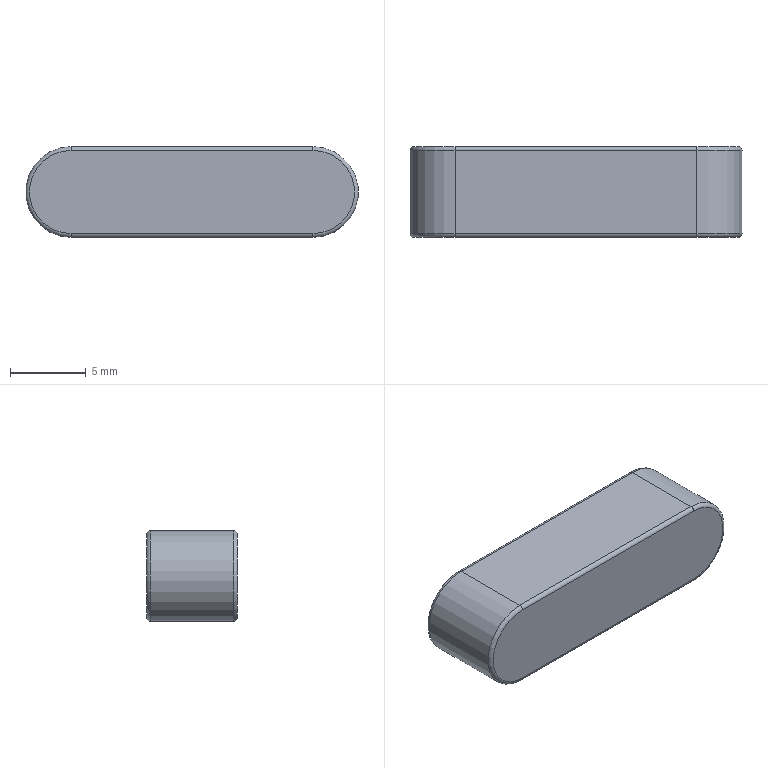Part | SolidWorks | features Extrusion 1, Fillet 1 | 1 solid | 14 faces | box 22 x 6 x 6 mm | volume 744.291 mm3 | cylinder 6 | plane 4 | torus 4 | commonest cylinder face diameters 0.5 x4 6 x2
STEP:
#1=CARTESIAN_POINT('',(-16.,5.75,-3.));
#2=VERTEX_POINT('',#1);
#3=CARTESIAN_POINT('',(-16.,0.25,-3.));
#4=VERTEX_POINT('',#3);
#5=CARTESIAN_POINT('',(-16.,6.,-3.));
#6=DIRECTION('',(0.,-1.,0.));
#7=VECTOR('',#6,1000.);
#8=LINE('',#5,#7);
#9=EDGE_CURVE('',#2,#4,#8,.T.);
#10=ORIENTED_EDGE('',*,*,#9,.T.);
#11=CARTESIAN_POINT('',(-16.,0.25,3.));
#12=VERTEX_POINT('',#11);
#13=CARTESIAN_POINT('',(-16.,0.25,0.));
#14=DIRECTION('',(0.,1.,0.));
#15=DIRECTION('',(0.,0.,1.));
#16=AXIS2_PLACEMENT_3D('',#13,#14,#15);
#17=CIRCLE('',#16,3.);
#18=EDGE_CURVE('',#4,#12,#17,.T.);
#19=ORIENTED_EDGE('',*,*,#18,.T.);
#20=CARTESIAN_POINT('',(-16.,5.75,3.));
#21=VERTEX_POINT('',#20);
#22=CARTESIAN_POINT('',(-16.,6.,3.));
#23=DIRECTION('',(0.,-1.,0.));
#24=VECTOR('',#23,1000.);
#25=LINE('',#22,#24);
#26=EDGE_CURVE('',#21,#12,#25,.T.);
#27=ORIENTED_EDGE('',*,*,#26,.F.);
#28=CARTESIAN_POINT('',(-16.,5.75,0.));
#29=DIRECTION('',(0.,-1.,0.));
#30=DIRECTION('',(0.,0.,1.));
#31=AXIS2_PLACEMENT_3D('',#28,#29,#30);
#32=CIRCLE('',#31,3.);
#33=EDGE_CURVE('',#21,#2,#32,.T.);
#34=ORIENTED_EDGE('',*,*,#33,.T.);
#35=EDGE_LOOP('',(#10,#19,#27,#34));
#36=FACE_OUTER_BOUND('',#35,.T.);
#37=CARTESIAN_POINT('',(-16.,6.,0.));
#38=DIRECTION('',(0.,-1.,0.));
#39=DIRECTION('',(0.,0.,-1.));
#40=AXIS2_PLACEMENT_3D('',#37,#38,#39);
#41=CYLINDRICAL_SURFACE('',#40,3.);
#42=ADVANCED_FACE('',(#36),#41,.T.);
#43=ORIENTED_EDGE('',*,*,#26,.T.);
#44=CARTESIAN_POINT('',(0.,0.25,3.));
#45=VERTEX_POINT('',#44);
#46=CARTESIAN_POINT('',(-16.,0.25,3.));
#47=DIRECTION('',(1.,0.,0.));
#48=VECTOR('',#47,1000.);
#49=LINE('',#46,#48);
#50=EDGE_CURVE('',#12,#45,#49,.T.);
#51=ORIENTED_EDGE('',*,*,#50,.T.);
#52=CARTESIAN_POINT('',(0.,5.75,3.));
#53=VERTEX_POINT('',#52);
#54=CARTESIAN_POINT('',(0.,6.,3.));
#55=DIRECTION('',(0.,-1.,0.));
#56=VECTOR('',#55,1000.);
#57=LINE('',#54,#56);
#58=EDGE_CURVE('',#53,#45,#57,.T.);
#59=ORIENTED_EDGE('',*,*,#58,.F.);
#60=CARTESIAN_POINT('',(-16.,5.75,3.));
#61=DIRECTION('',(-1.,0.,0.));
#62=VECTOR('',#61,1000.);
#63=LINE('',#60,#62);
#64=EDGE_CURVE('',#53,#21,#63,.T.);
#65=ORIENTED_EDGE('',*,*,#64,.T.);
#66=EDGE_LOOP('',(#43,#51,#59,#65));
#67=FACE_OUTER_BOUND('',#66,.T.);
#68=CARTESIAN_POINT('',(-16.,6.,3.));
#69=DIRECTION('',(0.,0.,-1.));
#70=DIRECTION('',(-1.,0.,0.));
#71=AXIS2_PLACEMENT_3D('',#68,#69,#70);
#72=PLANE('',#71);
#73=ADVANCED_FACE('',(#67),#72,.F.);
#74=ORIENTED_EDGE('',*,*,#58,.T.);
#75=CARTESIAN_POINT('',(0.,0.25,-3.));
#76=VERTEX_POINT('',#75);
#77=CARTESIAN_POINT('',(0.,0.25,0.));
#78=DIRECTION('',(0.,1.,0.));
#79=DIRECTION('',(0.,0.,1.));
#80=AXIS2_PLACEMENT_3D('',#77,#78,#79);
#81=CIRCLE('',#80,3.);
#82=EDGE_CURVE('',#45,#76,#81,.T.);
#83=ORIENTED_EDGE('',*,*,#82,.T.);
#84=CARTESIAN_POINT('',(0.,5.75,-3.));
#85=VERTEX_POINT('',#84);
#86=CARTESIAN_POINT('',(0.,6.,-3.));
#87=DIRECTION('',(0.,-1.,0.));
#88=VECTOR('',#87,1000.);
#89=LINE('',#86,#88);
#90=EDGE_CURVE('',#85,#76,#89,.T.);
#91=ORIENTED_EDGE('',*,*,#90,.F.);
#92=CARTESIAN_POINT('',(0.,5.75,0.));
#93=DIRECTION('',(0.,-1.,0.));
#94=DIRECTION('',(0.,0.,1.));
#95=AXIS2_PLACEMENT_3D('',#92,#93,#94);
#96=CIRCLE('',#95,3.);
#97=EDGE_CURVE('',#85,#53,#96,.T.);
#98=ORIENTED_EDGE('',*,*,#97,.T.);
#99=EDGE_LOOP('',(#74,#83,#91,#98));
#100=FACE_OUTER_BOUND('',#99,.T.);
#101=CARTESIAN_POINT('',(0.,6.,0.));
#102=DIRECTION('',(0.,-1.,0.));
#103=DIRECTION('',(0.,0.,-1.));
#104=AXIS2_PLACEMENT_3D('',#101,#102,#103);
#105=CYLINDRICAL_SURFACE('',#104,3.);
#106=ADVANCED_FACE('',(#100),#105,.T.);
#107=ORIENTED_EDGE('',*,*,#90,.T.);
#108=CARTESIAN_POINT('',(-16.,0.25,-3.));
#109=DIRECTION('',(-1.,0.,0.));
#110=VECTOR('',#109,1000.);
#111=LINE('',#108,#110);
#112=EDGE_CURVE('',#76,#4,#111,.T.);
#113=ORIENTED_EDGE('',*,*,#112,.T.);
#114=ORIENTED_EDGE('',*,*,#9,.F.);
#115=CARTESIAN_POINT('',(0.,5.75,-3.));
#116=DIRECTION('',(1.,0.,0.));
#117=VECTOR('',#116,1000.);
#118=LINE('',#115,#117);
#119=EDGE_CURVE('',#2,#85,#118,.T.);
#120=ORIENTED_EDGE('',*,*,#119,.T.);
#121=EDGE_LOOP('',(#107,#113,#114,#120));
#122=FACE_OUTER_BOUND('',#121,.T.);
#123=CARTESIAN_POINT('',(-16.,6.,-3.));
#124=DIRECTION('',(0.,0.,1.));
#125=DIRECTION('',(1.,0.,0.));
#126=AXIS2_PLACEMENT_3D('',#123,#124,#125);
#127=PLANE('',#126);
#128=ADVANCED_FACE('',(#122),#127,.F.);
#129=CARTESIAN_POINT('',(-16.,6.,2.75));
#130=VERTEX_POINT('',#129);
#131=CARTESIAN_POINT('',(0.,6.,2.75));
#132=VERTEX_POINT('',#131);
#133=CARTESIAN_POINT('',(0.,6.,2.75));
#134=DIRECTION('',(1.,0.,0.));
#135=VECTOR('',#134,1000.);
#136=LINE('',#133,#135);
#137=EDGE_CURVE('',#130,#132,#136,.T.);
#138=ORIENTED_EDGE('',*,*,#137,.T.);
#139=CARTESIAN_POINT('',(0.,6.,-2.75));
#140=VERTEX_POINT('',#139);
#141=CARTESIAN_POINT('',(0.,6.,0.));
#142=DIRECTION('',(0.,1.,0.));
#143=DIRECTION('',(0.,0.,1.));
#144=AXIS2_PLACEMENT_3D('',#141,#142,#143);
#145=CIRCLE('',#144,2.75);
#146=EDGE_CURVE('',#132,#140,#145,.T.);
#147=ORIENTED_EDGE('',*,*,#146,.T.);
#148=CARTESIAN_POINT('',(-16.,6.,-2.75));
#149=VERTEX_POINT('',#148);
#150=CARTESIAN_POINT('',(-16.,6.,-2.75));
#151=DIRECTION('',(-1.,0.,0.));
#152=VECTOR('',#151,1000.);
#153=LINE('',#150,#152);
#154=EDGE_CURVE('',#140,#149,#153,.T.);
#155=ORIENTED_EDGE('',*,*,#154,.T.);
#156=CARTESIAN_POINT('',(-16.,6.,0.));
#157=DIRECTION('',(0.,1.,0.));
#158=DIRECTION('',(0.,0.,1.));
#159=AXIS2_PLACEMENT_3D('',#156,#157,#158);
#160=CIRCLE('',#159,2.75);
#161=EDGE_CURVE('',#149,#130,#160,.T.);
#162=ORIENTED_EDGE('',*,*,#161,.T.);
#163=EDGE_LOOP('',(#138,#147,#155,#162));
#164=FACE_OUTER_BOUND('',#163,.T.);
#165=CARTESIAN_POINT('',(-16.,6.,0.));
#166=DIRECTION('',(0.,1.,0.));
#167=DIRECTION('',(0.,0.,1.));
#168=AXIS2_PLACEMENT_3D('',#165,#166,#167);
#169=PLANE('',#168);
#170=ADVANCED_FACE('',(#164),#169,.T.);
#171=CARTESIAN_POINT('',(-16.,0.,2.75));
#172=VERTEX_POINT('',#171);
#173=CARTESIAN_POINT('',(-16.,0.,-2.75));
#174=VERTEX_POINT('',#173);
#175=CARTESIAN_POINT('',(-16.,0.,0.));
#176=DIRECTION('',(0.,-1.,0.));
#177=DIRECTION('',(0.,0.,1.));
#178=AXIS2_PLACEMENT_3D('',#175,#176,#177);
#179=CIRCLE('',#178,2.75);
#180=EDGE_CURVE('',#172,#174,#179,.T.);
#181=ORIENTED_EDGE('',*,*,#180,.T.);
#182=CARTESIAN_POINT('',(0.,0.,-2.75));
#183=VERTEX_POINT('',#182);
#184=CARTESIAN_POINT('',(-16.,0.,-2.75));
#185=DIRECTION('',(1.,0.,0.));
#186=VECTOR('',#185,1000.);
#187=LINE('',#184,#186);
#188=EDGE_CURVE('',#174,#183,#187,.T.);
#189=ORIENTED_EDGE('',*,*,#188,.T.);
#190=CARTESIAN_POINT('',(0.,0.,2.75));
#191=VERTEX_POINT('',#190);
#192=CARTESIAN_POINT('',(0.,0.,0.));
#193=DIRECTION('',(0.,-1.,0.));
#194=DIRECTION('',(0.,0.,1.));
#195=AXIS2_PLACEMENT_3D('',#192,#193,#194);
#196=CIRCLE('',#195,2.75);
#197=EDGE_CURVE('',#183,#191,#196,.T.);
#198=ORIENTED_EDGE('',*,*,#197,.T.);
#199=CARTESIAN_POINT('',(-16.,0.,2.75));
#200=DIRECTION('',(-1.,0.,0.));
#201=VECTOR('',#200,1000.);
#202=LINE('',#199,#201);
#203=EDGE_CURVE('',#191,#172,#202,.T.);
#204=ORIENTED_EDGE('',*,*,#203,.T.);
#205=EDGE_LOOP('',(#181,#189,#198,#204));
#206=FACE_OUTER_BOUND('',#205,.T.);
#207=CARTESIAN_POINT('',(-16.,0.,0.));
#208=DIRECTION('',(0.,1.,0.));
#209=DIRECTION('',(0.,0.,1.));
#210=AXIS2_PLACEMENT_3D('',#207,#208,#209);
#211=PLANE('',#210);
#212=ADVANCED_FACE('',(#206),#211,.F.);
#213=CARTESIAN_POINT('',(-16.,0.25,2.75));
#214=DIRECTION('',(-1.,0.,0.));
#215=DIRECTION('',(0.,0.,1.));
#216=AXIS2_PLACEMENT_3D('',#213,#214,#215);
#217=CIRCLE('',#216,0.25);
#218=EDGE_CURVE('',#172,#12,#217,.T.);
#219=ORIENTED_EDGE('',*,*,#218,.F.);
#220=ORIENTED_EDGE('',*,*,#203,.F.);
#221=CARTESIAN_POINT('',(0.,0.25,2.75));
#222=DIRECTION('',(1.,0.,0.));
#223=DIRECTION('',(0.,0.,-1.));
#224=AXIS2_PLACEMENT_3D('',#221,#222,#223);
#225=CIRCLE('',#224,0.25);
#226=EDGE_CURVE('',#45,#191,#225,.T.);
#227=ORIENTED_EDGE('',*,*,#226,.F.);
#228=ORIENTED_EDGE('',*,*,#50,.F.);
#229=EDGE_LOOP('',(#219,#220,#227,#228));
#230=FACE_OUTER_BOUND('',#229,.T.);
#231=CARTESIAN_POINT('',(-16.,0.25,2.75));
#232=DIRECTION('',(1.,0.,0.));
#233=DIRECTION('',(0.,0.,-1.));
#234=AXIS2_PLACEMENT_3D('',#231,#232,#233);
#235=CYLINDRICAL_SURFACE('',#234,0.25);
#236=ADVANCED_FACE('',(#230),#235,.T.);
#237=ORIENTED_EDGE('',*,*,#226,.T.);
#238=ORIENTED_EDGE('',*,*,#197,.F.);
#239=CARTESIAN_POINT('',(0.,0.25,-2.75));
#240=DIRECTION('',(-1.,0.,0.));
#241=DIRECTION('',(0.,-1.,0.));
#242=AXIS2_PLACEMENT_3D('',#239,#240,#241);
#243=CIRCLE('',#242,0.25);
#244=EDGE_CURVE('',#76,#183,#243,.T.);
#245=ORIENTED_EDGE('',*,*,#244,.F.);
#246=ORIENTED_EDGE('',*,*,#82,.F.);
#247=EDGE_LOOP('',(#237,#238,#245,#246));
#248=FACE_OUTER_BOUND('',#247,.T.);
#249=CARTESIAN_POINT('',(0.,0.25,0.));
#250=DIRECTION('',(0.,1.,0.));
#251=DIRECTION('',(0.,0.,1.));
#252=AXIS2_PLACEMENT_3D('',#249,#250,#251);
#253=TOROIDAL_SURFACE('',#252,2.75,0.25);
#254=ADVANCED_FACE('',(#248),#253,.T.);
#255=ORIENTED_EDGE('',*,*,#218,.T.);
#256=ORIENTED_EDGE('',*,*,#18,.F.);
#257=CARTESIAN_POINT('',(-16.,0.25,-2.75));
#258=DIRECTION('',(1.,0.,0.));
#259=DIRECTION('',(0.,0.,-1.));
#260=AXIS2_PLACEMENT_3D('',#257,#258,#259);
#261=CIRCLE('',#260,0.25);
#262=EDGE_CURVE('',#174,#4,#261,.T.);
#263=ORIENTED_EDGE('',*,*,#262,.F.);
#264=ORIENTED_EDGE('',*,*,#180,.F.);
#265=EDGE_LOOP('',(#255,#256,#263,#264));
#266=FACE_OUTER_BOUND('',#265,.T.);
#267=CARTESIAN_POINT('',(-16.,0.25,0.));
#268=DIRECTION('',(0.,1.,0.));
#269=DIRECTION('',(0.,0.,1.));
#270=AXIS2_PLACEMENT_3D('',#267,#268,#269);
#271=TOROIDAL_SURFACE('',#270,2.75,0.25);
#272=ADVANCED_FACE('',(#266),#271,.T.);
#273=ORIENTED_EDGE('',*,*,#244,.T.);
#274=ORIENTED_EDGE('',*,*,#188,.F.);
#275=ORIENTED_EDGE('',*,*,#262,.T.);
#276=ORIENTED_EDGE('',*,*,#112,.F.);
#277=EDGE_LOOP('',(#273,#274,#275,#276));
#278=FACE_OUTER_BOUND('',#277,.T.);
#279=CARTESIAN_POINT('',(-16.,0.25,-2.75));
#280=DIRECTION('',(-1.,0.,0.));
#281=DIRECTION('',(0.,0.,1.));
#282=AXIS2_PLACEMENT_3D('',#279,#280,#281);
#283=CYLINDRICAL_SURFACE('',#282,0.25);
#284=ADVANCED_FACE('',(#278),#283,.T.);
#285=CARTESIAN_POINT('',(-16.,5.75,-2.75));
#286=DIRECTION('',(1.,0.,0.));
#287=DIRECTION('',(0.,0.,-1.));
#288=AXIS2_PLACEMENT_3D('',#285,#286,#287);
#289=CIRCLE('',#288,0.25);
#290=EDGE_CURVE('',#2,#149,#289,.T.);
#291=ORIENTED_EDGE('',*,*,#290,.F.);
#292=ORIENTED_EDGE('',*,*,#33,.F.);
#293=CARTESIAN_POINT('',(-16.,5.75,2.75));
#294=DIRECTION('',(1.,0.,0.));
#295=DIRECTION('',(0.,0.,-1.));
#296=AXIS2_PLACEMENT_3D('',#293,#294,#295);
#297=CIRCLE('',#296,0.25);
#298=EDGE_CURVE('',#130,#21,#297,.T.);
#299=ORIENTED_EDGE('',*,*,#298,.F.);
#300=ORIENTED_EDGE('',*,*,#161,.F.);
#301=EDGE_LOOP('',(#291,#292,#299,#300));
#302=FACE_OUTER_BOUND('',#301,.T.);
#303=CARTESIAN_POINT('',(-16.,5.75,0.));
#304=DIRECTION('',(0.,1.,0.));
#305=DIRECTION('',(0.,0.,1.));
#306=AXIS2_PLACEMENT_3D('',#303,#304,#305);
#307=TOROIDAL_SURFACE('',#306,2.75,0.25);
#308=ADVANCED_FACE('',(#302),#307,.T.);
#309=ORIENTED_EDGE('',*,*,#298,.T.);
#310=ORIENTED_EDGE('',*,*,#64,.F.);
#311=CARTESIAN_POINT('',(0.,5.75,2.75));
#312=DIRECTION('',(1.,0.,0.));
#313=DIRECTION('',(0.,0.,-1.));
#314=AXIS2_PLACEMENT_3D('',#311,#312,#313);
#315=CIRCLE('',#314,0.25);
#316=EDGE_CURVE('',#132,#53,#315,.T.);
#317=ORIENTED_EDGE('',*,*,#316,.F.);
#318=ORIENTED_EDGE('',*,*,#137,.F.);
#319=EDGE_LOOP('',(#309,#310,#317,#318));
#320=FACE_OUTER_BOUND('',#319,.T.);
#321=CARTESIAN_POINT('',(-16.,5.75,2.75));
#322=DIRECTION('',(-1.,0.,0.));
#323=DIRECTION('',(0.,0.,1.));
#324=AXIS2_PLACEMENT_3D('',#321,#322,#323);
#325=CYLINDRICAL_SURFACE('',#324,0.25);
#326=ADVANCED_FACE('',(#320),#325,.T.);
#327=ORIENTED_EDGE('',*,*,#290,.T.);
#328=ORIENTED_EDGE('',*,*,#154,.F.);
#329=CARTESIAN_POINT('',(0.,5.75,-2.75));
#330=DIRECTION('',(1.,0.,0.));
#331=DIRECTION('',(0.,0.,-1.));
#332=AXIS2_PLACEMENT_3D('',#329,#330,#331);
#333=CIRCLE('',#332,0.25);
#334=EDGE_CURVE('',#85,#140,#333,.T.);
#335=ORIENTED_EDGE('',*,*,#334,.F.);
#336=ORIENTED_EDGE('',*,*,#119,.F.);
#337=EDGE_LOOP('',(#327,#328,#335,#336));
#338=FACE_OUTER_BOUND('',#337,.T.);
#339=CARTESIAN_POINT('',(-16.,5.75,-2.75));
#340=DIRECTION('',(1.,0.,0.));
#341=DIRECTION('',(0.,0.,-1.));
#342=AXIS2_PLACEMENT_3D('',#339,#340,#341);
#343=CYLINDRICAL_SURFACE('',#342,0.25);
#344=ADVANCED_FACE('',(#338),#343,.T.);
#345=ORIENTED_EDGE('',*,*,#316,.T.);
#346=ORIENTED_EDGE('',*,*,#97,.F.);
#347=ORIENTED_EDGE('',*,*,#334,.T.);
#348=ORIENTED_EDGE('',*,*,#146,.F.);
#349=EDGE_LOOP('',(#345,#346,#347,#348));
#350=FACE_OUTER_BOUND('',#349,.T.);
#351=CARTESIAN_POINT('',(0.,5.75,0.));
#352=DIRECTION('',(0.,1.,0.));
#353=DIRECTION('',(0.,0.,1.));
#354=AXIS2_PLACEMENT_3D('',#351,#352,#353);
#355=TOROIDAL_SURFACE('',#354,2.75,0.25);
#356=ADVANCED_FACE('',(#350),#355,.T.);
#357=CLOSED_SHELL('',(#42,#73,#106,#128,#170,#212,#236,#254,#272,#284,#308,#326,#344,#356));
#358=MANIFOLD_SOLID_BREP('',#357);
#359=CARTESIAN_POINT('',(0.,0.,0.));
#360=DIRECTION('',(0.,0.,1.));
#361=DIRECTION('',(1.,0.,0.));
#362=AXIS2_PLACEMENT_3D('',#359,#360,#361);
#363=(LENGTH_UNIT()NAMED_UNIT(*)SI_UNIT(.MILLI.,.METRE.));
#364=UNCERTAINTY_MEASURE_WITH_UNIT(LENGTH_MEASURE(0.00001),#363,'','');
#365=(NAMED_UNIT(*)PLANE_ANGLE_UNIT()SI_UNIT($,.RADIAN.));
#366=(NAMED_UNIT(*)SI_UNIT($,.STERADIAN.)SOLID_ANGLE_UNIT());
#367=(GEOMETRIC_REPRESENTATION_CONTEXT(3)GLOBAL_UNCERTAINTY_ASSIGNED_CONTEXT((#364))GLOBAL_UNIT_ASSIGNED_CONTEXT((#363,#365,#366))REPRESENTATION_CONTEXT('',''));
#368=ADVANCED_BREP_SHAPE_REPRESENTATION('',(#358,#362),#367);